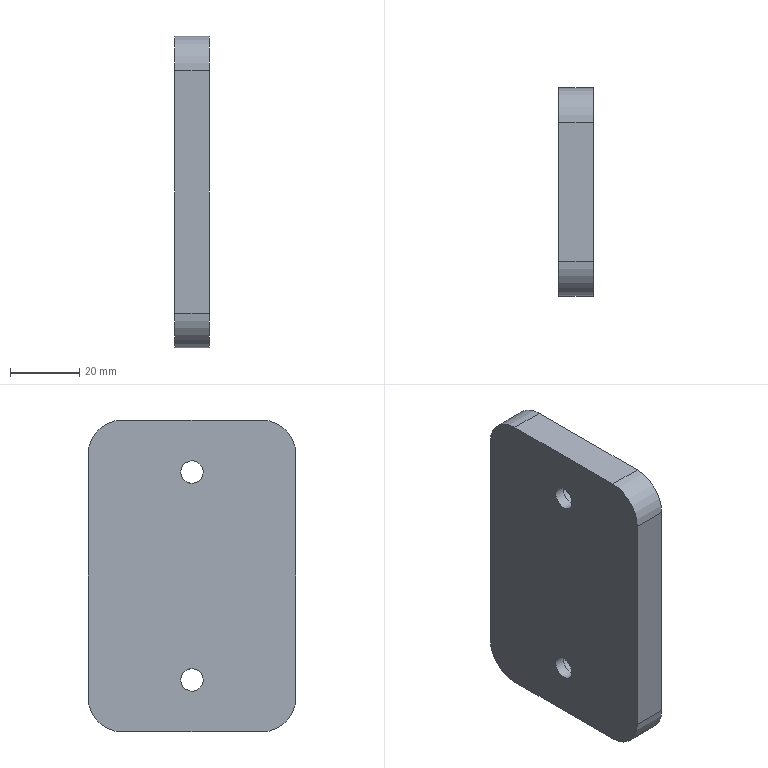Part | STEP file | solid 203 | 1 solid | 16 faces | box 10 x 60 x 90 mm | volume 51612 mm3 | plane 8 | cylinder 8 | commonest cylinder face diameters 20 x4 6.5 x2 11 x2